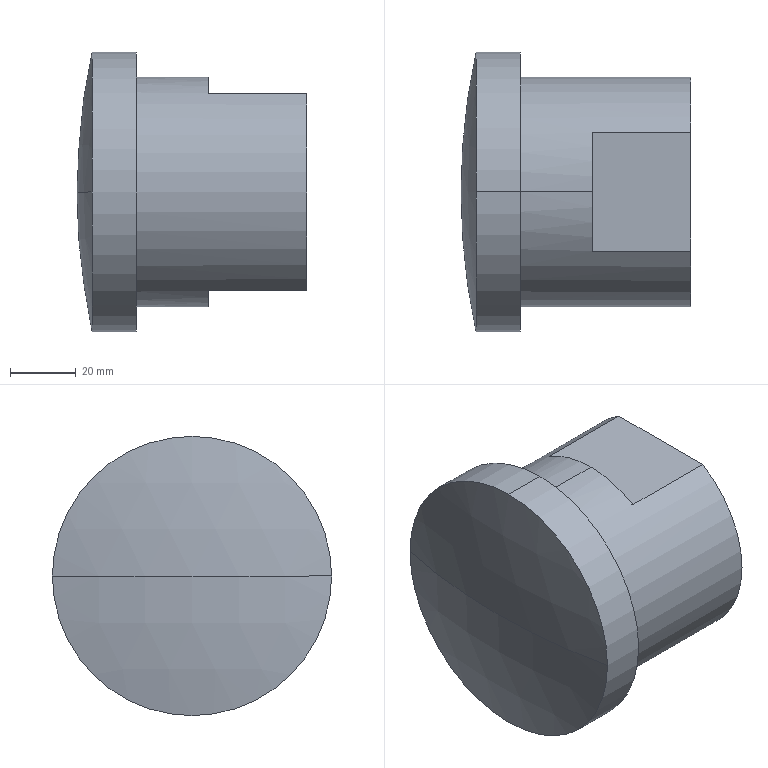Part | STEP file | OP10-027_cylinder connector (R) | 1 solid | 16 faces | box 70 x 85 x 85 mm | volume 228647 mm3 | cylinder 6 | plane 6 | cone 2 | sphere 2 | commonest cylinder face diameters 38.5 x2 70 x2 85 x2
STEP:
#1=CARTESIAN_POINT('',(0.,0.,0.));
#2=DIRECTION('',(0.,0.,1.));
#3=DIRECTION('',(1.,0.,0.));
#4=AXIS2_PLACEMENT_3D('',#1,#2,#3);
#5=CARTESIAN_POINT('',(-42.,0.,-19.25));
#6=VERTEX_POINT('',#5);
#7=CARTESIAN_POINT('',(0.,0.,-19.25));
#8=VERTEX_POINT('',#7);
#9=CARTESIAN_POINT('',(0.,0.,-19.25));
#10=DIRECTION('',(1.,0.,0.));
#11=VECTOR('',#10,1.);
#12=LINE('',#9,#11);
#13=CARTESIAN_POINT('',(0.,0.,0.));
#14=DIRECTION('',(1.,0.,0.));
#15=DIRECTION('',(0.,0.,-1.));
#16=AXIS2_PLACEMENT_3D('',#13,#14,#15);
#17=CYLINDRICAL_SURFACE('',#16,19.25);
#18=CARTESIAN_POINT('',(6.283,0.));
#19=DIRECTION('',(0.,1.));
#20=VECTOR('',#19,1.);
#21=LINE('',#18,#20);
#22=(GEOMETRIC_REPRESENTATION_CONTEXT(2)PARAMETRIC_REPRESENTATION_CONTEXT()REPRESENTATION_CONTEXT('',''));
#23=DEFINITIONAL_REPRESENTATION('',(#21),#22);
#24=PCURVE('',#17,#23);
#25=CARTESIAN_POINT('',(0.,0.,0.));
#26=DIRECTION('',(1.,0.,0.));
#27=DIRECTION('',(0.,0.,-1.));
#28=AXIS2_PLACEMENT_3D('',#25,#26,#27);
#29=CYLINDRICAL_SURFACE('',#28,19.25);
#30=CARTESIAN_POINT('',(0.,0.));
#31=DIRECTION('',(0.,1.));
#32=VECTOR('',#31,1.);
#33=LINE('',#30,#32);
#34=(GEOMETRIC_REPRESENTATION_CONTEXT(2)PARAMETRIC_REPRESENTATION_CONTEXT()REPRESENTATION_CONTEXT('',''));
#35=DEFINITIONAL_REPRESENTATION('',(#33),#34);
#36=PCURVE('',#29,#35);
#37=SURFACE_CURVE('',#12,(#24,#36),.PCURVE_S1.);
#38=EDGE_CURVE('',#6,#8,#37,.T.);
#39=ORIENTED_EDGE('',*,*,#38,.T.);
#40=CARTESIAN_POINT('',(0.,0.,19.25));
#41=VERTEX_POINT('',#40);
#42=CARTESIAN_POINT('',(0.,0.,0.));
#43=DIRECTION('',(1.,0.,0.));
#44=DIRECTION('',(0.,0.,-1.));
#45=AXIS2_PLACEMENT_3D('',#42,#43,#44);
#46=CIRCLE('',#45,19.25);
#47=CARTESIAN_POINT('',(0.,0.));
#48=DIRECTION('',(1.,0.));
#49=VECTOR('',#48,1.);
#50=LINE('',#47,#49);
#51=(GEOMETRIC_REPRESENTATION_CONTEXT(2)PARAMETRIC_REPRESENTATION_CONTEXT()REPRESENTATION_CONTEXT('',''));
#52=DEFINITIONAL_REPRESENTATION('',(#50),#51);
#53=PCURVE('',#17,#52);
#54=CARTESIAN_POINT('',(0.,0.,0.));
#55=DIRECTION('',(1.,0.,0.));
#56=DIRECTION('',(0.,0.,-1.));
#57=AXIS2_PLACEMENT_3D('',#54,#55,#56);
#58=PLANE('',#57);
#59=CARTESIAN_POINT('',(0.,0.));
#60=DIRECTION('',(1.,0.));
#61=AXIS2_PLACEMENT_2D('',#59,#60);
#62=CIRCLE('',#61,19.25);
#63=(GEOMETRIC_REPRESENTATION_CONTEXT(2)PARAMETRIC_REPRESENTATION_CONTEXT()REPRESENTATION_CONTEXT('',''));
#64=DEFINITIONAL_REPRESENTATION('',(#62),#63);
#65=PCURVE('',#58,#64);
#66=SURFACE_CURVE('',#46,(#53,#65),.PCURVE_S1.);
#67=EDGE_CURVE('',#41,#8,#66,.T.);
#68=ORIENTED_EDGE('',*,*,#67,.F.);
#69=CARTESIAN_POINT('',(-42.,0.,19.25));
#70=VERTEX_POINT('',#69);
#71=CARTESIAN_POINT('',(0.,0.,19.25));
#72=DIRECTION('',(1.,0.,0.));
#73=VECTOR('',#72,1.);
#74=LINE('',#71,#73);
#75=CARTESIAN_POINT('',(3.142,0.));
#76=DIRECTION('',(0.,1.));
#77=VECTOR('',#76,1.);
#78=LINE('',#75,#77);
#79=(GEOMETRIC_REPRESENTATION_CONTEXT(2)PARAMETRIC_REPRESENTATION_CONTEXT()REPRESENTATION_CONTEXT('',''));
#80=DEFINITIONAL_REPRESENTATION('',(#78),#79);
#81=PCURVE('',#17,#80);
#82=CARTESIAN_POINT('',(3.142,0.));
#83=DIRECTION('',(0.,1.));
#84=VECTOR('',#83,1.);
#85=LINE('',#82,#84);
#86=(GEOMETRIC_REPRESENTATION_CONTEXT(2)PARAMETRIC_REPRESENTATION_CONTEXT()REPRESENTATION_CONTEXT('',''));
#87=DEFINITIONAL_REPRESENTATION('',(#85),#86);
#88=PCURVE('',#29,#87);
#89=SURFACE_CURVE('',#74,(#81,#88),.PCURVE_S1.);
#90=EDGE_CURVE('',#70,#41,#89,.T.);
#91=ORIENTED_EDGE('',*,*,#90,.F.);
#92=CARTESIAN_POINT('',(-42.,0.,0.));
#93=DIRECTION('',(1.,0.,0.));
#94=DIRECTION('',(0.,0.,-1.));
#95=AXIS2_PLACEMENT_3D('',#92,#93,#94);
#96=CIRCLE('',#95,19.25);
#97=CARTESIAN_POINT('',(0.,-42.));
#98=DIRECTION('',(1.,0.));
#99=VECTOR('',#98,1.);
#100=LINE('',#97,#99);
#101=(GEOMETRIC_REPRESENTATION_CONTEXT(2)PARAMETRIC_REPRESENTATION_CONTEXT()REPRESENTATION_CONTEXT('',''));
#102=DEFINITIONAL_REPRESENTATION('',(#100),#101);
#103=PCURVE('',#17,#102);
#104=CARTESIAN_POINT('',(-42.,0.,0.));
#105=DIRECTION('',(1.,0.,0.));
#106=DIRECTION('',(0.,0.,-1.));
#107=AXIS2_PLACEMENT_3D('',#104,#105,#106);
#108=CONICAL_SURFACE('',#107,19.25,1.03);
#109=CARTESIAN_POINT('',(0.,0.));
#110=DIRECTION('',(1.,0.));
#111=VECTOR('',#110,1.);
#112=LINE('',#109,#111);
#113=(GEOMETRIC_REPRESENTATION_CONTEXT(2)PARAMETRIC_REPRESENTATION_CONTEXT()REPRESENTATION_CONTEXT('',''));
#114=DEFINITIONAL_REPRESENTATION('',(#112),#113);
#115=PCURVE('',#108,#114);
#116=SURFACE_CURVE('',#96,(#103,#115),.PCURVE_S1.);
#117=EDGE_CURVE('',#70,#6,#116,.T.);
#118=ORIENTED_EDGE('',*,*,#117,.T.);
#119=EDGE_LOOP('',(#39,#68,#91,#118));
#120=FACE_BOUND('',#119,.F.);
#121=ADVANCED_FACE('',(#120),#17,.F.);
#122=ORIENTED_EDGE('',*,*,#117,.F.);
#123=CARTESIAN_POINT('',(-53.567,0.,0.));
#124=VERTEX_POINT('',#123);
#125=CARTESIAN_POINT('',(-42.,0.,19.25));
#126=DIRECTION('',(0.515,0.,0.8572));
#127=VECTOR('',#126,1.);
#128=LINE('',#125,#127);
#129=CARTESIAN_POINT('',(3.142,0.));
#130=DIRECTION('',(0.,1.));
#131=VECTOR('',#130,1.);
#132=LINE('',#129,#131);
#133=(GEOMETRIC_REPRESENTATION_CONTEXT(2)PARAMETRIC_REPRESENTATION_CONTEXT()REPRESENTATION_CONTEXT('',''));
#134=DEFINITIONAL_REPRESENTATION('',(#132),#133);
#135=PCURVE('',#108,#134);
#136=CARTESIAN_POINT('',(-42.,0.,0.));
#137=DIRECTION('',(1.,0.,0.));
#138=DIRECTION('',(0.,0.,-1.));
#139=AXIS2_PLACEMENT_3D('',#136,#137,#138);
#140=CONICAL_SURFACE('',#139,19.25,1.03);
#141=CARTESIAN_POINT('',(3.142,0.));
#142=DIRECTION('',(0.,1.));
#143=VECTOR('',#142,1.);
#144=LINE('',#141,#143);
#145=(GEOMETRIC_REPRESENTATION_CONTEXT(2)PARAMETRIC_REPRESENTATION_CONTEXT()REPRESENTATION_CONTEXT('',''));
#146=DEFINITIONAL_REPRESENTATION('',(#144),#145);
#147=PCURVE('',#140,#146);
#148=SURFACE_CURVE('',#128,(#135,#147),.PCURVE_S1.);
#149=EDGE_CURVE('',#124,#70,#148,.T.);
#150=ORIENTED_EDGE('',*,*,#149,.F.);
#151=CARTESIAN_POINT('',(-42.,0.,-19.25));
#152=DIRECTION('',(0.515,0.,-0.8572));
#153=VECTOR('',#152,1.);
#154=LINE('',#151,#153);
#155=CARTESIAN_POINT('',(6.283,0.));
#156=DIRECTION('',(0.,1.));
#157=VECTOR('',#156,1.);
#158=LINE('',#155,#157);
#159=(GEOMETRIC_REPRESENTATION_CONTEXT(2)PARAMETRIC_REPRESENTATION_CONTEXT()REPRESENTATION_CONTEXT('',''));
#160=DEFINITIONAL_REPRESENTATION('',(#158),#159);
#161=PCURVE('',#108,#160);
#162=CARTESIAN_POINT('',(0.,0.));
#163=DIRECTION('',(0.,1.));
#164=VECTOR('',#163,1.);
#165=LINE('',#162,#164);
#166=(GEOMETRIC_REPRESENTATION_CONTEXT(2)PARAMETRIC_REPRESENTATION_CONTEXT()REPRESENTATION_CONTEXT('',''));
#167=DEFINITIONAL_REPRESENTATION('',(#165),#166);
#168=PCURVE('',#140,#167);
#169=SURFACE_CURVE('',#154,(#161,#168),.PCURVE_S1.);
#170=EDGE_CURVE('',#124,#6,#169,.T.);
#171=ORIENTED_EDGE('',*,*,#170,.T.);
#172=EDGE_LOOP('',(#122,#150,#171));
#173=FACE_BOUND('',#172,.F.);
#174=ADVANCED_FACE('',(#173),#108,.F.);
#175=CARTESIAN_POINT('',(-70.,0.,0.));
#176=VERTEX_POINT('',#175);
#177=CARTESIAN_POINT('',(-65.432,42.5,0.));
#178=VERTEX_POINT('',#177);
#179=CARTESIAN_POINT('',(130.,0.,0.));
#180=DIRECTION('',(0.,0.,-1.));
#181=DIRECTION('',(-1.,0.,0.));
#182=AXIS2_PLACEMENT_3D('',#179,#180,#181);
#183=CIRCLE('',#182,200.);
#184=CARTESIAN_POINT('',(130.,0.,0.));
#185=DIRECTION('',(0.,0.,1.));
#186=DIRECTION('',(0.,1.,0.));
#187=AXIS2_PLACEMENT_3D('',#184,#185,#186);
#188=SPHERICAL_SURFACE('',#187,200.);
#189=CARTESIAN_POINT('',(1.571,0.));
#190=DIRECTION('',(-1.,0.));
#191=VECTOR('',#190,1.);
#192=LINE('',#189,#191);
#193=(GEOMETRIC_REPRESENTATION_CONTEXT(2)PARAMETRIC_REPRESENTATION_CONTEXT()REPRESENTATION_CONTEXT('',''));
#194=DEFINITIONAL_REPRESENTATION('',(#192),#193);
#195=PCURVE('',#188,#194);
#196=CARTESIAN_POINT('',(130.,0.,0.));
#197=DIRECTION('',(0.,0.,1.));
#198=DIRECTION('',(0.,1.,0.));
#199=AXIS2_PLACEMENT_3D('',#196,#197,#198);
#200=SPHERICAL_SURFACE('',#199,200.);
#201=CARTESIAN_POINT('',(1.571,0.));
#202=DIRECTION('',(-1.,0.));
#203=VECTOR('',#202,1.);
#204=LINE('',#201,#203);
#205=(GEOMETRIC_REPRESENTATION_CONTEXT(2)PARAMETRIC_REPRESENTATION_CONTEXT()REPRESENTATION_CONTEXT('',''));
#206=DEFINITIONAL_REPRESENTATION('',(#204),#205);
#207=PCURVE('',#200,#206);
#208=SURFACE_CURVE('',#183,(#195,#207),.PCURVE_S1.);
#209=EDGE_CURVE('',#176,#178,#208,.T.);
#210=ORIENTED_EDGE('',*,*,#209,.F.);
#211=CARTESIAN_POINT('',(-65.432,-42.5,0.));
#212=VERTEX_POINT('',#211);
#213=CARTESIAN_POINT('',(130.,0.,0.));
#214=DIRECTION('',(0.,0.,1.));
#215=DIRECTION('',(0.,-1.,0.));
#216=AXIS2_PLACEMENT_3D('',#213,#214,#215);
#217=CIRCLE('',#216,200.);
#218=CARTESIAN_POINT('',(-3.142,0.));
#219=DIRECTION('',(1.,0.));
#220=VECTOR('',#219,1.);
#221=LINE('',#218,#220);
#222=(GEOMETRIC_REPRESENTATION_CONTEXT(2)PARAMETRIC_REPRESENTATION_CONTEXT()REPRESENTATION_CONTEXT('',''));
#223=DEFINITIONAL_REPRESENTATION('',(#221),#222);
#224=PCURVE('',#188,#223);
#225=CARTESIAN_POINT('',(-3.142,0.));
#226=DIRECTION('',(1.,0.));
#227=VECTOR('',#226,1.);
#228=LINE('',#225,#227);
#229=(GEOMETRIC_REPRESENTATION_CONTEXT(2)PARAMETRIC_REPRESENTATION_CONTEXT()REPRESENTATION_CONTEXT('',''));
#230=DEFINITIONAL_REPRESENTATION('',(#228),#229);
#231=PCURVE('',#200,#230);
#232=SURFACE_CURVE('',#217,(#224,#231),.PCURVE_S1.);
#233=EDGE_CURVE('',#176,#212,#232,.T.);
#234=ORIENTED_EDGE('',*,*,#233,.T.);
#235=CARTESIAN_POINT('',(-65.432,0.,42.5));
#236=VERTEX_POINT('',#235);
#237=CARTESIAN_POINT('',(-65.432,0.,0.));
#238=DIRECTION('',(1.,0.,0.));
#239=DIRECTION('',(0.,0.,-1.));
#240=AXIS2_PLACEMENT_3D('',#237,#238,#239);
#241=CIRCLE('',#240,42.5);
#242=CARTESIAN_POINT('',(1.571,0.2141));
#243=CARTESIAN_POINT('',(1.576,0.2141));
#244=CARTESIAN_POINT('',(1.586,0.2138));
#245=CARTESIAN_POINT('',(1.602,0.2121));
#246=CARTESIAN_POINT('',(1.617,0.2093));
#247=CARTESIAN_POINT('',(1.632,0.2055));
#248=CARTESIAN_POINT('',(1.647,0.2006));
#249=CARTESIAN_POINT('',(1.661,0.1947));
#250=CARTESIAN_POINT('',(1.675,0.1878));
#251=CARTESIAN_POINT('',(1.688,0.1799));
#252=CARTESIAN_POINT('',(1.701,0.1711));
#253=CARTESIAN_POINT('',(1.712,0.1614));
#254=CARTESIAN_POINT('',(1.724,0.151));
#255=CARTESIAN_POINT('',(1.734,0.1397));
#256=CARTESIAN_POINT('',(1.743,0.1278));
#257=CARTESIAN_POINT('',(1.752,0.1152));
#258=CARTESIAN_POINT('',(1.76,0.1021));
#259=CARTESIAN_POINT('',(1.766,0.08846));
#260=CARTESIAN_POINT('',(1.772,0.07439));
#261=CARTESIAN_POINT('',(1.777,0.05995));
#262=CARTESIAN_POINT('',(1.78,0.04522));
#263=CARTESIAN_POINT('',(1.783,0.03027));
#264=CARTESIAN_POINT('',(1.785,0.01517));
#265=CARTESIAN_POINT('',(1.785,0.005058));
#266=CARTESIAN_POINT('',(1.785,0.));
#267=B_SPLINE_CURVE_WITH_KNOTS('',3,(#242,#243,#244,#245,#246,#247,#248,#249,#250,#251,#252,#253,#254,#255,#256,#257,#258,#259,#260,#261,#262,#263,#264,#265,#266),.UNSPECIFIED.,.F.,.F.,(4,1,1,1,1,1,1,1,1,1,1,1,1,1,1,1,1,1,1,1,1,1,4),(3.142,3.213,3.284,3.356,3.427,3.499,3.57,3.641,3.713,3.784,3.856,3.927,3.998,4.07,4.141,4.213,4.284,4.355,4.427,4.498,4.57,4.641,4.712),.QUASI_UNIFORM_KNOTS.);
#268=(GEOMETRIC_REPRESENTATION_CONTEXT(2)PARAMETRIC_REPRESENTATION_CONTEXT()REPRESENTATION_CONTEXT('',''));
#269=DEFINITIONAL_REPRESENTATION('',(#267),#268);
#270=PCURVE('',#188,#269);
#271=CARTESIAN_POINT('',(0.,0.,0.));
#272=DIRECTION('',(1.,0.,0.));
#273=DIRECTION('',(0.,0.,-1.));
#274=AXIS2_PLACEMENT_3D('',#271,#272,#273);
#275=CYLINDRICAL_SURFACE('',#274,42.5);
#276=CARTESIAN_POINT('',(0.,-65.432));
#277=DIRECTION('',(1.,0.));
#278=VECTOR('',#277,1.);
#279=LINE('',#276,#278);
#280=(GEOMETRIC_REPRESENTATION_CONTEXT(2)PARAMETRIC_REPRESENTATION_CONTEXT()REPRESENTATION_CONTEXT('',''));
#281=DEFINITIONAL_REPRESENTATION('',(#279),#280);
#282=PCURVE('',#275,#281);
#283=SURFACE_CURVE('',#241,(#270,#282),.PCURVE_S1.);
#284=EDGE_CURVE('',#236,#212,#283,.T.);
#285=ORIENTED_EDGE('',*,*,#284,.F.);
#286=CARTESIAN_POINT('',(-65.432,0.,0.));
#287=DIRECTION('',(1.,0.,0.));
#288=DIRECTION('',(0.,0.,-1.));
#289=AXIS2_PLACEMENT_3D('',#286,#287,#288);
#290=CIRCLE('',#289,42.5);
#291=CARTESIAN_POINT('',(1.357,0.));
#292=CARTESIAN_POINT('',(1.357,0.005058));
#293=CARTESIAN_POINT('',(1.357,0.01517));
#294=CARTESIAN_POINT('',(1.359,0.03027));
#295=CARTESIAN_POINT('',(1.361,0.04522));
#296=CARTESIAN_POINT('',(1.365,0.05995));
#297=CARTESIAN_POINT('',(1.37,0.07439));
#298=CARTESIAN_POINT('',(1.375,0.08846));
#299=CARTESIAN_POINT('',(1.382,0.1021));
#300=CARTESIAN_POINT('',(1.39,0.1152));
#301=CARTESIAN_POINT('',(1.398,0.1278));
#302=CARTESIAN_POINT('',(1.408,0.1397));
#303=CARTESIAN_POINT('',(1.418,0.151));
#304=CARTESIAN_POINT('',(1.429,0.1614));
#305=CARTESIAN_POINT('',(1.441,0.1711));
#306=CARTESIAN_POINT('',(1.454,0.1799));
#307=CARTESIAN_POINT('',(1.467,0.1878));
#308=CARTESIAN_POINT('',(1.481,0.1947));
#309=CARTESIAN_POINT('',(1.495,0.2006));
#310=CARTESIAN_POINT('',(1.51,0.2055));
#311=CARTESIAN_POINT('',(1.525,0.2093));
#312=CARTESIAN_POINT('',(1.54,0.2121));
#313=CARTESIAN_POINT('',(1.555,0.2138));
#314=CARTESIAN_POINT('',(1.566,0.2141));
#315=CARTESIAN_POINT('',(1.571,0.2141));
#316=B_SPLINE_CURVE_WITH_KNOTS('',3,(#291,#292,#293,#294,#295,#296,#297,#298,#299,#300,#301,#302,#303,#304,#305,#306,#307,#308,#309,#310,#311,#312,#313,#314,#315),.UNSPECIFIED.,.F.,.F.,(4,1,1,1,1,1,1,1,1,1,1,1,1,1,1,1,1,1,1,1,1,1,4),(1.571,1.642,1.714,1.785,1.856,1.928,1.999,2.071,2.142,2.213,2.285,2.356,2.428,2.499,2.57,2.642,2.713,2.785,2.856,2.927,2.999,3.07,3.142),.QUASI_UNIFORM_KNOTS.);
#317=(GEOMETRIC_REPRESENTATION_CONTEXT(2)PARAMETRIC_REPRESENTATION_CONTEXT()REPRESENTATION_CONTEXT('',''));
#318=DEFINITIONAL_REPRESENTATION('',(#316),#317);
#319=PCURVE('',#188,#318);
#320=CARTESIAN_POINT('',(0.,0.,0.));
#321=DIRECTION('',(1.,0.,0.));
#322=DIRECTION('',(0.,0.,-1.));
#323=AXIS2_PLACEMENT_3D('',#320,#321,#322);
#324=CYLINDRICAL_SURFACE('',#323,42.5);
#325=CARTESIAN_POINT('',(0.,-65.432));
#326=DIRECTION('',(1.,0.));
#327=VECTOR('',#326,1.);
#328=LINE('',#325,#327);
#329=(GEOMETRIC_REPRESENTATION_CONTEXT(2)PARAMETRIC_REPRESENTATION_CONTEXT()REPRESENTATION_CONTEXT('',''));
#330=DEFINITIONAL_REPRESENTATION('',(#328),#329);
#331=PCURVE('',#324,#330);
#332=SURFACE_CURVE('',#290,(#319,#331),.PCURVE_S1.);
#333=EDGE_CURVE('',#178,#236,#332,.T.);
#334=ORIENTED_EDGE('',*,*,#333,.F.);
#335=EDGE_LOOP('',(#210,#234,#285,#334));
#336=FACE_BOUND('',#335,.T.);
#337=ADVANCED_FACE('',(#336),#188,.T.);
#338=CARTESIAN_POINT('',(-65.432,0.,-42.5));
#339=VERTEX_POINT('',#338);
#340=CARTESIAN_POINT('',(-65.432,0.,0.));
#341=DIRECTION('',(1.,0.,0.));
#342=DIRECTION('',(0.,0.,-1.));
#343=AXIS2_PLACEMENT_3D('',#340,#341,#342);
#344=CIRCLE('',#343,42.5);
#345=CARTESIAN_POINT('',(0.,-65.432));
#346=DIRECTION('',(1.,0.));
#347=VECTOR('',#346,1.);
#348=LINE('',#345,#347);
#349=(GEOMETRIC_REPRESENTATION_CONTEXT(2)PARAMETRIC_REPRESENTATION_CONTEXT()REPRESENTATION_CONTEXT('',''));
#350=DEFINITIONAL_REPRESENTATION('',(#348),#349);
#351=PCURVE('',#324,#350);
#352=CARTESIAN_POINT('',(1.571,-0.2141));
#353=CARTESIAN_POINT('',(1.566,-0.2141));
#354=CARTESIAN_POINT('',(1.555,-0.2138));
#355=CARTESIAN_POINT('',(1.54,-0.2121));
#356=CARTESIAN_POINT('',(1.525,-0.2093));
#357=CARTESIAN_POINT('',(1.51,-0.2055));
#358=CARTESIAN_POINT('',(1.495,-0.2006));
#359=CARTESIAN_POINT('',(1.481,-0.1947));
#360=CARTESIAN_POINT('',(1.467,-0.1878));
#361=CARTESIAN_POINT('',(1.454,-0.1799));
#362=CARTESIAN_POINT('',(1.441,-0.1711));
#363=CARTESIAN_POINT('',(1.429,-0.1614));
#364=CARTESIAN_POINT('',(1.418,-0.151));
#365=CARTESIAN_POINT('',(1.408,-0.1397));
#366=CARTESIAN_POINT('',(1.398,-0.1278));
#367=CARTESIAN_POINT('',(1.39,-0.1152));
#368=CARTESIAN_POINT('',(1.382,-0.1021));
#369=CARTESIAN_POINT('',(1.375,-0.08846));
#370=CARTESIAN_POINT('',(1.37,-0.07439));
#371=CARTESIAN_POINT('',(1.365,-0.05995));
#372=CARTESIAN_POINT('',(1.361,-0.04522));
#373=CARTESIAN_POINT('',(1.359,-0.03027));
#374=CARTESIAN_POINT('',(1.357,-0.01517));
#375=CARTESIAN_POINT('',(1.357,-0.005058));
#376=CARTESIAN_POINT('',(1.357,0.));
#377=B_SPLINE_CURVE_WITH_KNOTS('',3,(#352,#353,#354,#355,#356,#357,#358,#359,#360,#361,#362,#363,#364,#365,#366,#367,#368,#369,#370,#371,#372,#373,#374,#375,#376),.UNSPECIFIED.,.F.,.F.,(4,1,1,1,1,1,1,1,1,1,1,1,1,1,1,1,1,1,1,1,1,1,4),(0.,0.0714,0.1428,0.2142,0.2856,0.357,0.4284,0.4998,0.5712,0.6426,0.714,0.7854,0.8568,0.9282,0.9996,1.071,1.142,1.214,1.285,1.357,1.428,1.499,1.571),.QUASI_UNIFORM_KNOTS.);
#378=(GEOMETRIC_REPRESENTATION_CONTEXT(2)PARAMETRIC_REPRESENTATION_CONTEXT()REPRESENTATION_CONTEXT('',''));
#379=DEFINITIONAL_REPRESENTATION('',(#377),#378);
#380=PCURVE('',#200,#379);
#381=SURFACE_CURVE('',#344,(#351,#380),.PCURVE_S1.);
#382=EDGE_CURVE('',#339,#178,#381,.T.);
#383=ORIENTED_EDGE('',*,*,#382,.T.);
#384=ORIENTED_EDGE('',*,*,#333,.T.);
#385=CARTESIAN_POINT('',(-52.,0.,42.5));
#386=VERTEX_POINT('',#385);
#387=CARTESIAN_POINT('',(0.,0.,42.5));
#388=DIRECTION('',(1.,0.,0.));
#389=VECTOR('',#388,1.);
#390=LINE('',#387,#389);
#391=CARTESIAN_POINT('',(3.142,0.));
#392=DIRECTION('',(0.,1.));
#393=VECTOR('',#392,1.);
#394=LINE('',#391,#393);
#395=(GEOMETRIC_REPRESENTATION_CONTEXT(2)PARAMETRIC_REPRESENTATION_CONTEXT()REPRESENTATION_CONTEXT('',''));
#396=DEFINITIONAL_REPRESENTATION('',(#394),#395);
#397=PCURVE('',#324,#396);
#398=CARTESIAN_POINT('',(3.142,0.));
#399=DIRECTION('',(0.,1.));
#400=VECTOR('',#399,1.);
#401=LINE('',#398,#400);
#402=(GEOMETRIC_REPRESENTATION_CONTEXT(2)PARAMETRIC_REPRESENTATION_CONTEXT()REPRESENTATION_CONTEXT('',''));
#403=DEFINITIONAL_REPRESENTATION('',(#401),#402);
#404=PCURVE('',#275,#403);
#405=SURFACE_CURVE('',#390,(#397,#404),.PCURVE_S1.);
#406=EDGE_CURVE('',#236,#386,#405,.T.);
#407=ORIENTED_EDGE('',*,*,#406,.T.);
#408=CARTESIAN_POINT('',(-52.,0.,-42.5));
#409=VERTEX_POINT('',#408);
#410=CARTESIAN_POINT('',(-52.,0.,0.));
#411=DIRECTION('',(1.,0.,0.));
#412=DIRECTION('',(0.,0.,-1.));
#413=AXIS2_PLACEMENT_3D('',#410,#411,#412);
#414=CIRCLE('',#413,42.5);
#415=CARTESIAN_POINT('',(0.,-52.));
#416=DIRECTION('',(1.,0.));
#417=VECTOR('',#416,1.);
#418=LINE('',#415,#417);
#419=(GEOMETRIC_REPRESENTATION_CONTEXT(2)PARAMETRIC_REPRESENTATION_CONTEXT()REPRESENTATION_CONTEXT('',''));
#420=DEFINITIONAL_REPRESENTATION('',(#418),#419);
#421=PCURVE('',#324,#420);
#422=CARTESIAN_POINT('',(-52.,35.,0.));
#423=DIRECTION('',(1.,0.,0.));
#424=DIRECTION('',(0.,0.,-1.));
#425=AXIS2_PLACEMENT_3D('',#422,#423,#424);
#426=PLANE('',#425);
#427=CARTESIAN_POINT('',(0.,-35.));
#428=DIRECTION('',(1.,0.));
#429=AXIS2_PLACEMENT_2D('',#427,#428);
#430=CIRCLE('',#429,42.5);
#431=(GEOMETRIC_REPRESENTATION_CONTEXT(2)PARAMETRIC_REPRESENTATION_CONTEXT()REPRESENTATION_CONTEXT('',''));
#432=DEFINITIONAL_REPRESENTATION('',(#430),#431);
#433=PCURVE('',#426,#432);
#434=SURFACE_CURVE('',#414,(#421,#433),.PCURVE_S1.);
#435=EDGE_CURVE('',#409,#386,#434,.T.);
#436=ORIENTED_EDGE('',*,*,#435,.F.);
#437=CARTESIAN_POINT('',(0.,0.,-42.5));
#438=DIRECTION('',(1.,0.,0.));
#439=VECTOR('',#438,1.);
#440=LINE('',#437,#439);
#441=CARTESIAN_POINT('',(0.,0.));
#442=DIRECTION('',(0.,1.));
#443=VECTOR('',#442,1.);
#444=LINE('',#441,#443);
#445=(GEOMETRIC_REPRESENTATION_CONTEXT(2)PARAMETRIC_REPRESENTATION_CONTEXT()REPRESENTATION_CONTEXT('',''));
#446=DEFINITIONAL_REPRESENTATION('',(#444),#445);
#447=PCURVE('',#324,#446);
#448=CARTESIAN_POINT('',(6.283,0.));
#449=DIRECTION('',(0.,1.));
#450=VECTOR('',#449,1.);
#451=LINE('',#448,#450);
#452=(GEOMETRIC_REPRESENTATION_CONTEXT(2)PARAMETRIC_REPRESENTATION_CONTEXT()REPRESENTATION_CONTEXT('',''));
#453=DEFINITIONAL_REPRESENTATION('',(#451),#452);
#454=PCURVE('',#275,#453);
#455=SURFACE_CURVE('',#440,(#447,#454),.PCURVE_S1.);
#456=EDGE_CURVE('',#339,#409,#455,.T.);
#457=ORIENTED_EDGE('',*,*,#456,.F.);
#458=EDGE_LOOP('',(#383,#384,#407,#436,#457));
#459=FACE_BOUND('',#458,.T.);
#460=ADVANCED_FACE('',(#459),#324,.T.);
#461=CARTESIAN_POINT('',(-52.,0.,-35.));
#462=VERTEX_POINT('',#461);
#463=CARTESIAN_POINT('',(-52.,0.,35.));
#464=VERTEX_POINT('',#463);
#465=CARTESIAN_POINT('',(-52.,0.,0.));
#466=DIRECTION('',(1.,0.,0.));
#467=DIRECTION('',(0.,0.,-1.));
#468=AXIS2_PLACEMENT_3D('',#465,#466,#467);
#469=CIRCLE('',#468,35.);
#470=CARTESIAN_POINT('',(0.,0.,0.));
#471=DIRECTION('',(1.,0.,0.));
#472=DIRECTION('',(0.,0.,-1.));
#473=AXIS2_PLACEMENT_3D('',#470,#471,#472);
#474=CYLINDRICAL_SURFACE('',#473,35.);
#475=CARTESIAN_POINT('',(0.,-52.));
#476=DIRECTION('',(1.,0.));
#477=VECTOR('',#476,1.);
#478=LINE('',#475,#477);
#479=(GEOMETRIC_REPRESENTATION_CONTEXT(2)PARAMETRIC_REPRESENTATION_CONTEXT()REPRESENTATION_CONTEXT('',''));
#480=DEFINITIONAL_REPRESENTATION('',(#478),#479);
#481=PCURVE('',#474,#480);
#482=CARTESIAN_POINT('',(0.,-35.));
#483=DIRECTION('',(1.,0.));
#484=AXIS2_PLACEMENT_2D('',#482,#483);
#485=CIRCLE('',#484,35.);
#486=(GEOMETRIC_REPRESENTATION_CONTEXT(2)PARAMETRIC_REPRESENTATION_CONTEXT()REPRESENTATION_CONTEXT('',''));
#487=DEFINITIONAL_REPRESENTATION('',(#485),#486);
#488=PCURVE('',#426,#487);
#489=SURFACE_CURVE('',#469,(#481,#488),.PCURVE_S1.);
#490=EDGE_CURVE('',#462,#464,#489,.T.);
#491=ORIENTED_EDGE('',*,*,#490,.T.);
#492=CARTESIAN_POINT('',(-30.,0.,35.));
#493=VERTEX_POINT('',#492);
#494=CARTESIAN_POINT('',(0.,0.,35.));
#495=DIRECTION('',(1.,0.,0.));
#496=VECTOR('',#495,1.);
#497=LINE('',#494,#496);
#498=CARTESIAN_POINT('',(3.142,0.));
#499=DIRECTION('',(0.,1.));
#500=VECTOR('',#499,1.);
#501=LINE('',#498,#500);
#502=(GEOMETRIC_REPRESENTATION_CONTEXT(2)PARAMETRIC_REPRESENTATION_CONTEXT()REPRESENTATION_CONTEXT('',''));
#503=DEFINITIONAL_REPRESENTATION('',(#501),#502);
#504=PCURVE('',#474,#503);
#505=CARTESIAN_POINT('',(0.,0.,0.));
#506=DIRECTION('',(1.,0.,0.));
#507=DIRECTION('',(0.,0.,-1.));
#508=AXIS2_PLACEMENT_3D('',#505,#506,#507);
#509=CYLINDRICAL_SURFACE('',#508,35.);
#510=CARTESIAN_POINT('',(3.142,0.));
#511=DIRECTION('',(0.,1.));
#512=VECTOR('',#511,1.);
#513=LINE('',#510,#512);
#514=(GEOMETRIC_REPRESENTATION_CONTEXT(2)PARAMETRIC_REPRESENTATION_CONTEXT()REPRESENTATION_CONTEXT('',''));
#515=DEFINITIONAL_REPRESENTATION('',(#513),#514);
#516=PCURVE('',#509,#515);
#517=SURFACE_CURVE('',#497,(#504,#516),.PCURVE_S1.);
#518=EDGE_CURVE('',#464,#493,#517,.T.);
#519=ORIENTED_EDGE('',*,*,#518,.T.);
#520=CARTESIAN_POINT('',(-30.,18.028,30.));
#521=VERTEX_POINT('',#520);
#522=CARTESIAN_POINT('',(-30.,0.,0.));
#523=DIRECTION('',(-1.,0.,0.));
#524=DIRECTION('',(0.,0.,-1.));
#525=AXIS2_PLACEMENT_3D('',#522,#523,#524);
#526=CIRCLE('',#525,35.);
#527=CARTESIAN_POINT('',(6.283,-30.));
#528=DIRECTION('',(-1.,0.));
#529=VECTOR('',#528,1.);
#530=LINE('',#527,#529);
#531=(GEOMETRIC_REPRESENTATION_CONTEXT(2)PARAMETRIC_REPRESENTATION_CONTEXT()REPRESENTATION_CONTEXT('',''));
#532=DEFINITIONAL_REPRESENTATION('',(#530),#531);
#533=PCURVE('',#474,#532);
#534=CARTESIAN_POINT('',(-30.,-35.,40.));
#535=DIRECTION('',(1.,0.,0.));
#536=DIRECTION('',(0.,0.,-1.));
#537=AXIS2_PLACEMENT_3D('',#534,#535,#536);
#538=PLANE('',#537);
#539=CARTESIAN_POINT('',(75.,35.));
#540=CARTESIAN_POINT('',(75.,-25.622));
#541=CARTESIAN_POINT('',(22.5,4.689));
#542=CARTESIAN_POINT('',(-30.,35.));
#543=CARTESIAN_POINT('',(22.5,65.311));
#544=CARTESIAN_POINT('',(75.,95.622));
#545=CARTESIAN_POINT('',(75.,35.));
#546=(BOUNDED_CURVE()B_SPLINE_CURVE(2,(#539,#540,#541,#542,#543,#544,#545),.UNSPECIFIED.,.T.,.F.)B_SPLINE_CURVE_WITH_KNOTS((1,2,2,2,2,1),(-2.094,0.,2.094,4.189,6.283,8.378),.UNSPECIFIED.)CURVE()GEOMETRIC_REPRESENTATION_ITEM()RATIONAL_B_SPLINE_CURVE((1.,0.5,1.,0.5,1.,0.5,1.))REPRESENTATION_ITEM(''));
#547=(GEOMETRIC_REPRESENTATION_CONTEXT(2)PARAMETRIC_REPRESENTATION_CONTEXT()REPRESENTATION_CONTEXT('',''));
#548=DEFINITIONAL_REPRESENTATION('',(#546),#547);
#549=PCURVE('',#538,#548);
#550=SURFACE_CURVE('',#526,(#533,#549),.PCURVE_S1.);
#551=EDGE_CURVE('',#493,#521,#550,.T.);
#552=ORIENTED_EDGE('',*,*,#551,.T.);
#553=CARTESIAN_POINT('',(0.,18.028,30.));
#554=VERTEX_POINT('',#553);
#555=CARTESIAN_POINT('',(0.,18.028,30.));
#556=DIRECTION('',(-1.,0.,0.));
#557=VECTOR('',#556,1.);
#558=LINE('',#555,#557);
#559=CARTESIAN_POINT('',(2.6,0.));
#560=DIRECTION('',(0.,-1.));
#561=VECTOR('',#560,1.);
#562=LINE('',#559,#561);
#563=(GEOMETRIC_REPRESENTATION_CONTEXT(2)PARAMETRIC_REPRESENTATION_CONTEXT()REPRESENTATION_CONTEXT('',''));
#564=DEFINITIONAL_REPRESENTATION('',(#562),#563);
#565=PCURVE('',#474,#564);
#566=CARTESIAN_POINT('',(0.,0.,30.));
#567=DIRECTION('',(0.,0.,-1.));
#568=DIRECTION('',(-1.,0.,0.));
#569=AXIS2_PLACEMENT_3D('',#566,#567,#568);
#570=PLANE('',#569);
#571=CARTESIAN_POINT('',(0.,18.028));
#572=DIRECTION('',(1.,0.));
#573=VECTOR('',#572,1.);
#574=LINE('',#571,#573);
#575=(GEOMETRIC_REPRESENTATION_CONTEXT(2)PARAMETRIC_REPRESENTATION_CONTEXT()REPRESENTATION_CONTEXT('',''));
#576=DEFINITIONAL_REPRESENTATION('',(#574),#575);
#577=PCURVE('',#570,#576);
#578=SURFACE_CURVE('',#558,(#565,#577),.PCURVE_S1.);
#579=EDGE_CURVE('',#554,#521,#578,.T.);
#580=ORIENTED_EDGE('',*,*,#579,.F.);
#581=CARTESIAN_POINT('',(0.,18.028,-30.));
#582=VERTEX_POINT('',#581);
#583=CARTESIAN_POINT('',(0.,0.,0.));
#584=DIRECTION('',(1.,0.,0.));
#585=DIRECTION('',(0.,0.,-1.));
#586=AXIS2_PLACEMENT_3D('',#583,#584,#585);
#587=CIRCLE('',#586,35.);
#588=CARTESIAN_POINT('',(0.,0.));
#589=DIRECTION('',(1.,0.));
#590=VECTOR('',#589,1.);
#591=LINE('',#588,#590);
#592=(GEOMETRIC_REPRESENTATION_CONTEXT(2)PARAMETRIC_REPRESENTATION_CONTEXT()REPRESENTATION_CONTEXT('',''));
#593=DEFINITIONAL_REPRESENTATION('',(#591),#592);
#594=PCURVE('',#474,#593);
#595=CARTESIAN_POINT('',(0.,0.));
#596=DIRECTION('',(1.,0.));
#597=AXIS2_PLACEMENT_2D('',#595,#596);
#598=CIRCLE('',#597,35.);
#599=(GEOMETRIC_REPRESENTATION_CONTEXT(2)PARAMETRIC_REPRESENTATION_CONTEXT()REPRESENTATION_CONTEXT('',''));
#600=DEFINITIONAL_REPRESENTATION('',(#598),#599);
#601=PCURVE('',#58,#600);
#602=SURFACE_CURVE('',#587,(#594,#601),.PCURVE_S1.);
#603=EDGE_CURVE('',#582,#554,#602,.T.);
#604=ORIENTED_EDGE('',*,*,#603,.F.);
#605=CARTESIAN_POINT('',(-30.,18.028,-30.));
#606=VERTEX_POINT('',#605);
#607=CARTESIAN_POINT('',(0.,18.028,-30.));
#608=DIRECTION('',(1.,0.,0.));
#609=VECTOR('',#608,1.);
#610=LINE('',#607,#609);
#611=CARTESIAN_POINT('',(0.5411,0.));
#612=DIRECTION('',(0.,1.));
#613=VECTOR('',#612,1.);
#614=LINE('',#611,#613);
#615=(GEOMETRIC_REPRESENTATION_CONTEXT(2)PARAMETRIC_REPRESENTATION_CONTEXT()REPRESENTATION_CONTEXT('',''));
#616=DEFINITIONAL_REPRESENTATION('',(#614),#615);
#617=PCURVE('',#474,#616);
#618=CARTESIAN_POINT('',(0.,0.,-30.));
#619=DIRECTION('',(0.,0.,1.));
#620=DIRECTION('',(-1.,0.,0.));
#621=AXIS2_PLACEMENT_3D('',#618,#619,#620);
#622=PLANE('',#621);
#623=CARTESIAN_POINT('',(0.,-18.028));
#624=DIRECTION('',(-1.,0.));
#625=VECTOR('',#624,1.);
#626=LINE('',#623,#625);
#627=(GEOMETRIC_REPRESENTATION_CONTEXT(2)PARAMETRIC_REPRESENTATION_CONTEXT()REPRESENTATION_CONTEXT('',''));
#628=DEFINITIONAL_REPRESENTATION('',(#626),#627);
#629=PCURVE('',#622,#628);
#630=SURFACE_CURVE('',#610,(#617,#629),.PCURVE_S1.);
#631=EDGE_CURVE('',#606,#582,#630,.T.);
#632=ORIENTED_EDGE('',*,*,#631,.F.);
#633=CARTESIAN_POINT('',(-30.,0.,-35.));
#634=VERTEX_POINT('',#633);
#635=CARTESIAN_POINT('',(-30.,0.,0.));
#636=DIRECTION('',(1.,0.,0.));
#637=DIRECTION('',(0.,0.,1.));
#638=AXIS2_PLACEMENT_3D('',#635,#636,#637);
#639=CIRCLE('',#638,35.);
#640=CARTESIAN_POINT('',(-3.142,-30.));
#641=DIRECTION('',(1.,0.));
#642=VECTOR('',#641,1.);
#643=LINE('',#640,#642);
#644=(GEOMETRIC_REPRESENTATION_CONTEXT(2)PARAMETRIC_REPRESENTATION_CONTEXT()REPRESENTATION_CONTEXT('',''));
#645=DEFINITIONAL_REPRESENTATION('',(#643),#644);
#646=PCURVE('',#474,#645);
#647=CARTESIAN_POINT('',(-30.,-35.,-40.));
#648=DIRECTION('',(-1.,0.,0.));
#649=DIRECTION('',(0.,0.,1.));
#650=AXIS2_PLACEMENT_3D('',#647,#648,#649);
#651=PLANE('',#650);
#652=CARTESIAN_POINT('',(75.,35.));
#653=CARTESIAN_POINT('',(75.,-25.622));
#654=CARTESIAN_POINT('',(22.5,4.689));
#655=CARTESIAN_POINT('',(-30.,35.));
#656=CARTESIAN_POINT('',(22.5,65.311));
#657=CARTESIAN_POINT('',(75.,95.622));
#658=CARTESIAN_POINT('',(75.,35.));
#659=(BOUNDED_CURVE()B_SPLINE_CURVE(2,(#652,#653,#654,#655,#656,#657,#658),.UNSPECIFIED.,.T.,.F.)B_SPLINE_CURVE_WITH_KNOTS((1,2,2,2,2,1),(-2.094,0.,2.094,4.189,6.283,8.378),.UNSPECIFIED.)CURVE()GEOMETRIC_REPRESENTATION_ITEM()RATIONAL_B_SPLINE_CURVE((1.,0.5,1.,0.5,1.,0.5,1.))REPRESENTATION_ITEM(''));
#660=(GEOMETRIC_REPRESENTATION_CONTEXT(2)PARAMETRIC_REPRESENTATION_CONTEXT()REPRESENTATION_CONTEXT('',''));
#661=DEFINITIONAL_REPRESENTATION('',(#659),#660);
#662=PCURVE('',#651,#661);
#663=SURFACE_CURVE('',#639,(#646,#662),.PCURVE_S1.);
#664=EDGE_CURVE('',#634,#606,#663,.T.);
#665=ORIENTED_EDGE('',*,*,#664,.F.);
#666=CARTESIAN_POINT('',(0.,0.,-35.));
#667=DIRECTION('',(1.,0.,0.));
#668=VECTOR('',#667,1.);
#669=LINE('',#666,#668);
#670=CARTESIAN_POINT('',(0.,0.));
#671=DIRECTION('',(0.,1.));
#672=VECTOR('',#671,1.);
#673=LINE('',#670,#672);
#674=(GEOMETRIC_REPRESENTATION_CONTEXT(2)PARAMETRIC_REPRESENTATION_CONTEXT()REPRESENTATION_CONTEXT('',''));
#675=DEFINITIONAL_REPRESENTATION('',(#673),#674);
#676=PCURVE('',#474,#675);
#677=CARTESIAN_POINT('',(6.283,0.));
#678=DIRECTION('',(0.,1.));
#679=VECTOR('',#678,1.);
#680=LINE('',#677,#679);
#681=(GEOMETRIC_REPRESENTATION_CONTEXT(2)PARAMETRIC_REPRESENTATION_CONTEXT()REPRESENTATION_CONTEXT('',''));
#682=DEFINITIONAL_REPRESENTATION('',(#680),#681);
#683=PCURVE('',#509,#682);
#684=SURFACE_CURVE('',#669,(#676,#683),.PCURVE_S1.);
#685=EDGE_CURVE('',#462,#634,#684,.T.);
#686=ORIENTED_EDGE('',*,*,#685,.F.);
#687=EDGE_LOOP('',(#491,#519,#552,#580,#604,#632,#665,#686));
#688=FACE_BOUND('',#687,.T.);
#689=ADVANCED_FACE('',(#688),#474,.T.);
#690=CARTESIAN_POINT('',(0.,0.,0.));
#691=DIRECTION('',(1.,0.,0.));
#692=DIRECTION('',(0.,0.,-1.));
#693=AXIS2_PLACEMENT_3D('',#690,#691,#692);
#694=CIRCLE('',#693,19.25);
#695=CARTESIAN_POINT('',(0.,0.));
#696=DIRECTION('',(1.,0.));
#697=AXIS2_PLACEMENT_2D('',#695,#696);
#698=CIRCLE('',#697,19.25);
#699=(GEOMETRIC_REPRESENTATION_CONTEXT(2)PARAMETRIC_REPRESENTATION_CONTEXT()REPRESENTATION_CONTEXT('',''));
#700=DEFINITIONAL_REPRESENTATION('',(#698),#699);
#701=PCURVE('',#58,#700);
#702=CARTESIAN_POINT('',(0.,0.));
#703=DIRECTION('',(1.,0.));
#704=VECTOR('',#703,1.);
#705=LINE('',#702,#704);
#706=(GEOMETRIC_REPRESENTATION_CONTEXT(2)PARAMETRIC_REPRESENTATION_CONTEXT()REPRESENTATION_CONTEXT('',''));
#707=DEFINITIONAL_REPRESENTATION('',(#705),#706);
#708=PCURVE('',#29,#707);
#709=SURFACE_CURVE('',#694,(#701,#708),.PCURVE_S1.);
#710=EDGE_CURVE('',#8,#41,#709,.T.);
#711=ORIENTED_EDGE('',*,*,#710,.F.);
#712=ORIENTED_EDGE('',*,*,#67,.F.);
#713=EDGE_LOOP('',(#711,#712));
#714=FACE_BOUND('',#713,.T.);
#715=CARTESIAN_POINT('',(0.,-18.028,-30.));
#716=VERTEX_POINT('',#715);
#717=CARTESIAN_POINT('',(0.,0.,-30.));
#718=DIRECTION('',(0.,-1.,0.));
#719=VECTOR('',#718,1.);
#720=LINE('',#717,#719);
#721=CARTESIAN_POINT('',(30.,0.));
#722=DIRECTION('',(0.,-1.));
#723=VECTOR('',#722,1.);
#724=LINE('',#721,#723);
#725=(GEOMETRIC_REPRESENTATION_CONTEXT(2)PARAMETRIC_REPRESENTATION_CONTEXT()REPRESENTATION_CONTEXT('',''));
#726=DEFINITIONAL_REPRESENTATION('',(#724),#725);
#727=PCURVE('',#58,#726);
#728=CARTESIAN_POINT('',(0.,0.));
#729=DIRECTION('',(0.,1.));
#730=VECTOR('',#729,1.);
#731=LINE('',#728,#730);
#732=(GEOMETRIC_REPRESENTATION_CONTEXT(2)PARAMETRIC_REPRESENTATION_CONTEXT()REPRESENTATION_CONTEXT('',''));
#733=DEFINITIONAL_REPRESENTATION('',(#731),#732);
#734=PCURVE('',#622,#733);
#735=SURFACE_CURVE('',#720,(#727,#734),.PCURVE_S1.);
#736=EDGE_CURVE('',#582,#716,#735,.T.);
#737=ORIENTED_EDGE('',*,*,#736,.F.);
#738=ORIENTED_EDGE('',*,*,#603,.T.);
#739=CARTESIAN_POINT('',(0.,-18.028,30.));
#740=VERTEX_POINT('',#739);
#741=CARTESIAN_POINT('',(0.,0.,30.));
#742=DIRECTION('',(0.,1.,0.));
#743=VECTOR('',#742,1.);
#744=LINE('',#741,#743);
#745=CARTESIAN_POINT('',(-30.,0.));
#746=DIRECTION('',(0.,1.));
#747=VECTOR('',#746,1.);
#748=LINE('',#745,#747);
#749=(GEOMETRIC_REPRESENTATION_CONTEXT(2)PARAMETRIC_REPRESENTATION_CONTEXT()REPRESENTATION_CONTEXT('',''));
#750=DEFINITIONAL_REPRESENTATION('',(#748),#749);
#751=PCURVE('',#58,#750);
#752=CARTESIAN_POINT('',(0.,0.));
#753=DIRECTION('',(0.,1.));
#754=VECTOR('',#753,1.);
#755=LINE('',#752,#754);
#756=(GEOMETRIC_REPRESENTATION_CONTEXT(2)PARAMETRIC_REPRESENTATION_CONTEXT()REPRESENTATION_CONTEXT('',''));
#757=DEFINITIONAL_REPRESENTATION('',(#755),#756);
#758=PCURVE('',#570,#757);
#759=SURFACE_CURVE('',#744,(#751,#758),.PCURVE_S1.);
#760=EDGE_CURVE('',#740,#554,#759,.T.);
#761=ORIENTED_EDGE('',*,*,#760,.F.);
#762=CARTESIAN_POINT('',(0.,0.,0.));
#763=DIRECTION('',(1.,0.,0.));
#764=DIRECTION('',(0.,0.,-1.));
#765=AXIS2_PLACEMENT_3D('',#762,#763,#764);
#766=CIRCLE('',#765,35.);
#767=CARTESIAN_POINT('',(0.,0.));
#768=DIRECTION('',(1.,0.));
#769=AXIS2_PLACEMENT_2D('',#767,#768);
#770=CIRCLE('',#769,35.);
#771=(GEOMETRIC_REPRESENTATION_CONTEXT(2)PARAMETRIC_REPRESENTATION_CONTEXT()REPRESENTATION_CONTEXT('',''));
#772=DEFINITIONAL_REPRESENTATION('',(#770),#771);
#773=PCURVE('',#58,#772);
#774=CARTESIAN_POINT('',(0.,0.));
#775=DIRECTION('',(1.,0.));
#776=VECTOR('',#775,1.);
#777=LINE('',#774,#776);
#778=(GEOMETRIC_REPRESENTATION_CONTEXT(2)PARAMETRIC_REPRESENTATION_CONTEXT()REPRESENTATION_CONTEXT('',''));
#779=DEFINITIONAL_REPRESENTATION('',(#777),#778);
#780=PCURVE('',#509,#779);
#781=SURFACE_CURVE('',#766,(#773,#780),.PCURVE_S1.);
#782=EDGE_CURVE('',#740,#716,#781,.T.);
#783=ORIENTED_EDGE('',*,*,#782,.T.);
#784=EDGE_LOOP('',(#737,#738,#761,#783));
#785=FACE_BOUND('',#784,.T.);
#786=ADVANCED_FACE('',(#714,#785),#58,.T.);
#787=ORIENTED_EDGE('',*,*,#518,.F.);
#788=CARTESIAN_POINT('',(-52.,0.,0.));
#789=DIRECTION('',(1.,0.,0.));
#790=DIRECTION('',(0.,0.,-1.));
#791=AXIS2_PLACEMENT_3D('',#788,#789,#790);
#792=CIRCLE('',#791,35.);
#793=CARTESIAN_POINT('',(0.,-52.));
#794=DIRECTION('',(1.,0.));
#795=VECTOR('',#794,1.);
#796=LINE('',#793,#795);
#797=(GEOMETRIC_REPRESENTATION_CONTEXT(2)PARAMETRIC_REPRESENTATION_CONTEXT()REPRESENTATION_CONTEXT('',''));
#798=DEFINITIONAL_REPRESENTATION('',(#796),#797);
#799=PCURVE('',#509,#798);
#800=CARTESIAN_POINT('',(0.,-35.));
#801=DIRECTION('',(1.,0.));
#802=AXIS2_PLACEMENT_2D('',#800,#801);
#803=CIRCLE('',#802,35.);
#804=(GEOMETRIC_REPRESENTATION_CONTEXT(2)PARAMETRIC_REPRESENTATION_CONTEXT()REPRESENTATION_CONTEXT('',''));
#805=DEFINITIONAL_REPRESENTATION('',(#803),#804);
#806=PCURVE('',#426,#805);
#807=SURFACE_CURVE('',#792,(#799,#806),.PCURVE_S1.);
#808=EDGE_CURVE('',#464,#462,#807,.T.);
#809=ORIENTED_EDGE('',*,*,#808,.T.);
#810=ORIENTED_EDGE('',*,*,#685,.T.);
#811=CARTESIAN_POINT('',(-30.,-18.028,-30.));
#812=VERTEX_POINT('',#811);
#813=CARTESIAN_POINT('',(-30.,0.,0.));
#814=DIRECTION('',(1.,0.,0.));
#815=DIRECTION('',(0.,0.,1.));
#816=AXIS2_PLACEMENT_3D('',#813,#814,#815);
#817=CIRCLE('',#816,35.);
#818=CARTESIAN_POINT('',(3.142,-30.));
#819=DIRECTION('',(1.,0.));
#820=VECTOR('',#819,1.);
#821=LINE('',#818,#820);
#822=(GEOMETRIC_REPRESENTATION_CONTEXT(2)PARAMETRIC_REPRESENTATION_CONTEXT()REPRESENTATION_CONTEXT('',''));
#823=DEFINITIONAL_REPRESENTATION('',(#821),#822);
#824=PCURVE('',#509,#823);
#825=CARTESIAN_POINT('',(75.,35.));
#826=CARTESIAN_POINT('',(75.,-25.622));
#827=CARTESIAN_POINT('',(22.5,4.689));
#828=CARTESIAN_POINT('',(-30.,35.));
#829=CARTESIAN_POINT('',(22.5,65.311));
#830=CARTESIAN_POINT('',(75.,95.622));
#831=CARTESIAN_POINT('',(75.,35.));
#832=(BOUNDED_CURVE()B_SPLINE_CURVE(2,(#825,#826,#827,#828,#829,#830,#831),.UNSPECIFIED.,.T.,.F.)B_SPLINE_CURVE_WITH_KNOTS((1,2,2,2,2,1),(-2.094,0.,2.094,4.189,6.283,8.378),.UNSPECIFIED.)CURVE()GEOMETRIC_REPRESENTATION_ITEM()RATIONAL_B_SPLINE_CURVE((1.,0.5,1.,0.5,1.,0.5,1.))REPRESENTATION_ITEM(''));
#833=(GEOMETRIC_REPRESENTATION_CONTEXT(2)PARAMETRIC_REPRESENTATION_CONTEXT()REPRESENTATION_CONTEXT('',''));
#834=DEFINITIONAL_REPRESENTATION('',(#832),#833);
#835=PCURVE('',#651,#834);
#836=SURFACE_CURVE('',#817,(#824,#835),.PCURVE_S1.);
#837=EDGE_CURVE('',#812,#634,#836,.T.);
#838=ORIENTED_EDGE('',*,*,#837,.F.);
#839=CARTESIAN_POINT('',(0.,-18.028,-30.));
#840=DIRECTION('',(-1.,0.,0.));
#841=VECTOR('',#840,1.);
#842=LINE('',#839,#841);
#843=CARTESIAN_POINT('',(5.742,0.));
#844=DIRECTION('',(0.,-1.));
#845=VECTOR('',#844,1.);
#846=LINE('',#843,#845);
#847=(GEOMETRIC_REPRESENTATION_CONTEXT(2)PARAMETRIC_REPRESENTATION_CONTEXT()REPRESENTATION_CONTEXT('',''));
#848=DEFINITIONAL_REPRESENTATION('',(#846),#847);
#849=PCURVE('',#509,#848);
#850=CARTESIAN_POINT('',(0.,18.028));
#851=DIRECTION('',(1.,0.));
#852=VECTOR('',#851,1.);
#853=LINE('',#850,#852);
#854=(GEOMETRIC_REPRESENTATION_CONTEXT(2)PARAMETRIC_REPRESENTATION_CONTEXT()REPRESENTATION_CONTEXT('',''));
#855=DEFINITIONAL_REPRESENTATION('',(#853),#854);
#856=PCURVE('',#622,#855);
#857=SURFACE_CURVE('',#842,(#849,#856),.PCURVE_S1.);
#858=EDGE_CURVE('',#716,#812,#857,.T.);
#859=ORIENTED_EDGE('',*,*,#858,.F.);
#860=ORIENTED_EDGE('',*,*,#782,.F.);
#861=CARTESIAN_POINT('',(-30.,-18.028,30.));
#862=VERTEX_POINT('',#861);
#863=CARTESIAN_POINT('',(0.,-18.028,30.));
#864=DIRECTION('',(1.,0.,0.));
#865=VECTOR('',#864,1.);
#866=LINE('',#863,#865);
#867=CARTESIAN_POINT('',(3.683,0.));
#868=DIRECTION('',(0.,1.));
#869=VECTOR('',#868,1.);
#870=LINE('',#867,#869);
#871=(GEOMETRIC_REPRESENTATION_CONTEXT(2)PARAMETRIC_REPRESENTATION_CONTEXT()REPRESENTATION_CONTEXT('',''));
#872=DEFINITIONAL_REPRESENTATION('',(#870),#871);
#873=PCURVE('',#509,#872);
#874=CARTESIAN_POINT('',(0.,-18.028));
#875=DIRECTION('',(-1.,0.));
#876=VECTOR('',#875,1.);
#877=LINE('',#874,#876);
#878=(GEOMETRIC_REPRESENTATION_CONTEXT(2)PARAMETRIC_REPRESENTATION_CONTEXT()REPRESENTATION_CONTEXT('',''));
#879=DEFINITIONAL_REPRESENTATION('',(#877),#878);
#880=PCURVE('',#570,#879);
#881=SURFACE_CURVE('',#866,(#873,#880),.PCURVE_S1.);
#882=EDGE_CURVE('',#862,#740,#881,.T.);
#883=ORIENTED_EDGE('',*,*,#882,.F.);
#884=CARTESIAN_POINT('',(-30.,0.,0.));
#885=DIRECTION('',(-1.,0.,0.));
#886=DIRECTION('',(0.,0.,-1.));
#887=AXIS2_PLACEMENT_3D('',#884,#885,#886);
#888=CIRCLE('',#887,35.);
#889=CARTESIAN_POINT('',(6.283,-30.));
#890=DIRECTION('',(-1.,0.));
#891=VECTOR('',#890,1.);
#892=LINE('',#889,#891);
#893=(GEOMETRIC_REPRESENTATION_CONTEXT(2)PARAMETRIC_REPRESENTATION_CONTEXT()REPRESENTATION_CONTEXT('',''));
#894=DEFINITIONAL_REPRESENTATION('',(#892),#893);
#895=PCURVE('',#509,#894);
#896=CARTESIAN_POINT('',(75.,35.));
#897=CARTESIAN_POINT('',(75.,-25.622));
#898=CARTESIAN_POINT('',(22.5,4.689));
#899=CARTESIAN_POINT('',(-30.,35.));
#900=CARTESIAN_POINT('',(22.5,65.311));
#901=CARTESIAN_POINT('',(75.,95.622));
#902=CARTESIAN_POINT('',(75.,35.));
#903=(BOUNDED_CURVE()B_SPLINE_CURVE(2,(#896,#897,#898,#899,#900,#901,#902),.UNSPECIFIED.,.T.,.F.)B_SPLINE_CURVE_WITH_KNOTS((1,2,2,2,2,1),(-2.094,0.,2.094,4.189,6.283,8.378),.UNSPECIFIED.)CURVE()GEOMETRIC_REPRESENTATION_ITEM()RATIONAL_B_SPLINE_CURVE((1.,0.5,1.,0.5,1.,0.5,1.))REPRESENTATION_ITEM(''));
#904=(GEOMETRIC_REPRESENTATION_CONTEXT(2)PARAMETRIC_REPRESENTATION_CONTEXT()REPRESENTATION_CONTEXT('',''));
#905=DEFINITIONAL_REPRESENTATION('',(#903),#904);
#906=PCURVE('',#538,#905);
#907=SURFACE_CURVE('',#888,(#895,#906),.PCURVE_S1.);
#908=EDGE_CURVE('',#862,#493,#907,.T.);
#909=ORIENTED_EDGE('',*,*,#908,.T.);
#910=EDGE_LOOP('',(#787,#809,#810,#838,#859,#860,#883,#909));
#911=FACE_BOUND('',#910,.T.);
#912=ADVANCED_FACE('',(#911),#509,.T.);
#913=ORIENTED_EDGE('',*,*,#435,.T.);
#914=CARTESIAN_POINT('',(-52.,0.,0.));
#915=DIRECTION('',(1.,0.,0.));
#916=DIRECTION('',(0.,0.,-1.));
#917=AXIS2_PLACEMENT_3D('',#914,#915,#916);
#918=CIRCLE('',#917,42.5);
#919=CARTESIAN_POINT('',(0.,-35.));
#920=DIRECTION('',(1.,0.));
#921=AXIS2_PLACEMENT_2D('',#919,#920);
#922=CIRCLE('',#921,42.5);
#923=(GEOMETRIC_REPRESENTATION_CONTEXT(2)PARAMETRIC_REPRESENTATION_CONTEXT()REPRESENTATION_CONTEXT('',''));
#924=DEFINITIONAL_REPRESENTATION('',(#922),#923);
#925=PCURVE('',#426,#924);
#926=CARTESIAN_POINT('',(0.,-52.));
#927=DIRECTION('',(1.,0.));
#928=VECTOR('',#927,1.);
#929=LINE('',#926,#928);
#930=(GEOMETRIC_REPRESENTATION_CONTEXT(2)PARAMETRIC_REPRESENTATION_CONTEXT()REPRESENTATION_CONTEXT('',''));
#931=DEFINITIONAL_REPRESENTATION('',(#929),#930);
#932=PCURVE('',#275,#931);
#933=SURFACE_CURVE('',#918,(#925,#932),.PCURVE_S1.);
#934=EDGE_CURVE('',#386,#409,#933,.T.);
#935=ORIENTED_EDGE('',*,*,#934,.T.);
#936=EDGE_LOOP('',(#913,#935));
#937=FACE_BOUND('',#936,.T.);
#938=ORIENTED_EDGE('',*,*,#490,.F.);
#939=ORIENTED_EDGE('',*,*,#808,.F.);
#940=EDGE_LOOP('',(#938,#939));
#941=FACE_BOUND('',#940,.T.);
#942=ADVANCED_FACE('',(#937,#941),#426,.T.);
#943=ORIENTED_EDGE('',*,*,#406,.F.);
#944=ORIENTED_EDGE('',*,*,#284,.T.);
#945=CARTESIAN_POINT('',(-65.432,0.,0.));
#946=DIRECTION('',(1.,0.,0.));
#947=DIRECTION('',(0.,0.,-1.));
#948=AXIS2_PLACEMENT_3D('',#945,#946,#947);
#949=CIRCLE('',#948,42.5);
#950=CARTESIAN_POINT('',(0.,-65.432));
#951=DIRECTION('',(1.,0.));
#952=VECTOR('',#951,1.);
#953=LINE('',#950,#952);
#954=(GEOMETRIC_REPRESENTATION_CONTEXT(2)PARAMETRIC_REPRESENTATION_CONTEXT()REPRESENTATION_CONTEXT('',''));
#955=DEFINITIONAL_REPRESENTATION('',(#953),#954);
#956=PCURVE('',#275,#955);
#957=CARTESIAN_POINT('',(1.785,0.));
#958=CARTESIAN_POINT('',(1.785,-0.005058));
#959=CARTESIAN_POINT('',(1.785,-0.01517));
#960=CARTESIAN_POINT('',(1.783,-0.03027));
#961=CARTESIAN_POINT('',(1.78,-0.04522));
#962=CARTESIAN_POINT('',(1.777,-0.05995));
#963=CARTESIAN_POINT('',(1.772,-0.07439));
#964=CARTESIAN_POINT('',(1.766,-0.08846));
#965=CARTESIAN_POINT('',(1.76,-0.1021));
#966=CARTESIAN_POINT('',(1.752,-0.1152));
#967=CARTESIAN_POINT('',(1.743,-0.1278));
#968=CARTESIAN_POINT('',(1.734,-0.1397));
#969=CARTESIAN_POINT('',(1.724,-0.151));
#970=CARTESIAN_POINT('',(1.712,-0.1614));
#971=CARTESIAN_POINT('',(1.701,-0.1711));
#972=CARTESIAN_POINT('',(1.688,-0.1799));
#973=CARTESIAN_POINT('',(1.675,-0.1878));
#974=CARTESIAN_POINT('',(1.661,-0.1947));
#975=CARTESIAN_POINT('',(1.647,-0.2006));
#976=CARTESIAN_POINT('',(1.632,-0.2055));
#977=CARTESIAN_POINT('',(1.617,-0.2093));
#978=CARTESIAN_POINT('',(1.602,-0.2121));
#979=CARTESIAN_POINT('',(1.586,-0.2138));
#980=CARTESIAN_POINT('',(1.576,-0.2141));
#981=CARTESIAN_POINT('',(1.571,-0.2141));
#982=B_SPLINE_CURVE_WITH_KNOTS('',3,(#957,#958,#959,#960,#961,#962,#963,#964,#965,#966,#967,#968,#969,#970,#971,#972,#973,#974,#975,#976,#977,#978,#979,#980,#981),.UNSPECIFIED.,.F.,.F.,(4,1,1,1,1,1,1,1,1,1,1,1,1,1,1,1,1,1,1,1,1,1,4),(4.712,4.784,4.855,4.927,4.998,5.069,5.141,5.212,5.284,5.355,5.426,5.498,5.569,5.641,5.712,5.783,5.855,5.926,5.998,6.069,6.14,6.212,6.283),.QUASI_UNIFORM_KNOTS.);
#983=(GEOMETRIC_REPRESENTATION_CONTEXT(2)PARAMETRIC_REPRESENTATION_CONTEXT()REPRESENTATION_CONTEXT('',''));
#984=DEFINITIONAL_REPRESENTATION('',(#982),#983);
#985=PCURVE('',#200,#984);
#986=SURFACE_CURVE('',#949,(#956,#985),.PCURVE_S1.);
#987=EDGE_CURVE('',#212,#339,#986,.T.);
#988=ORIENTED_EDGE('',*,*,#987,.T.);
#989=ORIENTED_EDGE('',*,*,#456,.T.);
#990=ORIENTED_EDGE('',*,*,#934,.F.);
#991=EDGE_LOOP('',(#943,#944,#988,#989,#990));
#992=FACE_BOUND('',#991,.T.);
#993=ADVANCED_FACE('',(#992),#275,.T.);
#994=ORIENTED_EDGE('',*,*,#233,.F.);
#995=ORIENTED_EDGE('',*,*,#209,.T.);
#996=ORIENTED_EDGE('',*,*,#382,.F.);
#997=ORIENTED_EDGE('',*,*,#987,.F.);
#998=EDGE_LOOP('',(#994,#995,#996,#997));
#999=FACE_BOUND('',#998,.T.);
#1000=ADVANCED_FACE('',(#999),#200,.T.);
#1001=CARTESIAN_POINT('',(-30.,-35.,30.));
#1002=DIRECTION('',(0.,-1.,0.));
#1003=VECTOR('',#1002,1.);
#1004=LINE('',#1001,#1003);
#1005=CARTESIAN_POINT('',(10.,0.));
#1006=DIRECTION('',(0.,-1.));
#1007=VECTOR('',#1006,1.);
#1008=LINE('',#1005,#1007);
#1009=(GEOMETRIC_REPRESENTATION_CONTEXT(2)PARAMETRIC_REPRESENTATION_CONTEXT()REPRESENTATION_CONTEXT('',''));
#1010=DEFINITIONAL_REPRESENTATION('',(#1008),#1009);
#1011=PCURVE('',#538,#1010);
#1012=CARTESIAN_POINT('',(30.,-35.));
#1013=DIRECTION('',(0.,-1.));
#1014=VECTOR('',#1013,1.);
#1015=LINE('',#1012,#1014);
#1016=(GEOMETRIC_REPRESENTATION_CONTEXT(2)PARAMETRIC_REPRESENTATION_CONTEXT()REPRESENTATION_CONTEXT('',''));
#1017=DEFINITIONAL_REPRESENTATION('',(#1015),#1016);
#1018=PCURVE('',#570,#1017);
#1019=SURFACE_CURVE('',#1004,(#1011,#1018),.PCURVE_S1.);
#1020=EDGE_CURVE('',#521,#862,#1019,.T.);
#1021=ORIENTED_EDGE('',*,*,#1020,.F.);
#1022=ORIENTED_EDGE('',*,*,#551,.F.);
#1023=ORIENTED_EDGE('',*,*,#908,.F.);
#1024=EDGE_LOOP('',(#1021,#1022,#1023));
#1025=FACE_BOUND('',#1024,.T.);
#1026=ADVANCED_FACE('',(#1025),#538,.T.);
#1027=ORIENTED_EDGE('',*,*,#579,.T.);
#1028=ORIENTED_EDGE('',*,*,#1020,.T.);
#1029=ORIENTED_EDGE('',*,*,#882,.T.);
#1030=ORIENTED_EDGE('',*,*,#760,.T.);
#1031=EDGE_LOOP('',(#1027,#1028,#1029,#1030));
#1032=FACE_BOUND('',#1031,.T.);
#1033=ADVANCED_FACE('',(#1032),#570,.F.);
#1034=ORIENTED_EDGE('',*,*,#837,.T.);
#1035=ORIENTED_EDGE('',*,*,#664,.T.);
#1036=CARTESIAN_POINT('',(-30.,-35.,-30.));
#1037=DIRECTION('',(0.,-1.,0.));
#1038=VECTOR('',#1037,1.);
#1039=LINE('',#1036,#1038);
#1040=CARTESIAN_POINT('',(10.,0.));
#1041=DIRECTION('',(0.,-1.));
#1042=VECTOR('',#1041,1.);
#1043=LINE('',#1040,#1042);
#1044=(GEOMETRIC_REPRESENTATION_CONTEXT(2)PARAMETRIC_REPRESENTATION_CONTEXT()REPRESENTATION_CONTEXT('',''));
#1045=DEFINITIONAL_REPRESENTATION('',(#1043),#1044);
#1046=PCURVE('',#651,#1045);
#1047=CARTESIAN_POINT('',(30.,35.));
#1048=DIRECTION('',(0.,1.));
#1049=VECTOR('',#1048,1.);
#1050=LINE('',#1047,#1049);
#1051=(GEOMETRIC_REPRESENTATION_CONTEXT(2)PARAMETRIC_REPRESENTATION_CONTEXT()REPRESENTATION_CONTEXT('',''));
#1052=DEFINITIONAL_REPRESENTATION('',(#1050),#1051);
#1053=PCURVE('',#622,#1052);
#1054=SURFACE_CURVE('',#1039,(#1046,#1053),.PCURVE_S1.);
#1055=EDGE_CURVE('',#606,#812,#1054,.T.);
#1056=ORIENTED_EDGE('',*,*,#1055,.T.);
#1057=EDGE_LOOP('',(#1034,#1035,#1056));
#1058=FACE_BOUND('',#1057,.T.);
#1059=ADVANCED_FACE('',(#1058),#651,.F.);
#1060=ORIENTED_EDGE('',*,*,#858,.T.);
#1061=ORIENTED_EDGE('',*,*,#1055,.F.);
#1062=ORIENTED_EDGE('',*,*,#631,.T.);
#1063=ORIENTED_EDGE('',*,*,#736,.T.);
#1064=EDGE_LOOP('',(#1060,#1061,#1062,#1063));
#1065=FACE_BOUND('',#1064,.T.);
#1066=ADVANCED_FACE('',(#1065),#622,.F.);
#1067=CARTESIAN_POINT('',(-42.,0.,0.));
#1068=DIRECTION('',(1.,0.,0.));
#1069=DIRECTION('',(0.,0.,-1.));
#1070=AXIS2_PLACEMENT_3D('',#1067,#1068,#1069);
#1071=CIRCLE('',#1070,19.25);
#1072=CARTESIAN_POINT('',(0.,0.));
#1073=DIRECTION('',(1.,0.));
#1074=VECTOR('',#1073,1.);
#1075=LINE('',#1072,#1074);
#1076=(GEOMETRIC_REPRESENTATION_CONTEXT(2)PARAMETRIC_REPRESENTATION_CONTEXT()REPRESENTATION_CONTEXT('',''));
#1077=DEFINITIONAL_REPRESENTATION('',(#1075),#1076);
#1078=PCURVE('',#140,#1077);
#1079=CARTESIAN_POINT('',(0.,-42.));
#1080=DIRECTION('',(1.,0.));
#1081=VECTOR('',#1080,1.);
#1082=LINE('',#1079,#1081);
#1083=(GEOMETRIC_REPRESENTATION_CONTEXT(2)PARAMETRIC_REPRESENTATION_CONTEXT()REPRESENTATION_CONTEXT('',''));
#1084=DEFINITIONAL_REPRESENTATION('',(#1082),#1083);
#1085=PCURVE('',#29,#1084);
#1086=SURFACE_CURVE('',#1071,(#1078,#1085),.PCURVE_S1.);
#1087=EDGE_CURVE('',#6,#70,#1086,.T.);
#1088=ORIENTED_EDGE('',*,*,#1087,.F.);
#1089=ORIENTED_EDGE('',*,*,#170,.F.);
#1090=ORIENTED_EDGE('',*,*,#149,.T.);
#1091=EDGE_LOOP('',(#1088,#1089,#1090));
#1092=FACE_BOUND('',#1091,.F.);
#1093=ADVANCED_FACE('',(#1092),#140,.F.);
#1094=ORIENTED_EDGE('',*,*,#710,.F.);
#1095=ORIENTED_EDGE('',*,*,#38,.F.);
#1096=ORIENTED_EDGE('',*,*,#1087,.T.);
#1097=ORIENTED_EDGE('',*,*,#90,.T.);
#1098=EDGE_LOOP('',(#1094,#1095,#1096,#1097));
#1099=FACE_BOUND('',#1098,.F.);
#1100=ADVANCED_FACE('',(#1099),#29,.F.);
#1101=CLOSED_SHELL('',(#121,#174,#337,#460,#689,#786,#912,#942,#993,#1000,#1026,#1033,#1059,#1066,#1093,#1100));
#1102=MANIFOLD_SOLID_BREP('',#1101);
#1103=(LENGTH_UNIT()NAMED_UNIT(*)SI_UNIT(.MILLI.,.METRE.));
#1104=UNCERTAINTY_MEASURE_WITH_UNIT(LENGTH_MEASURE(0.0000001),#1103,'','');
#1105=(NAMED_UNIT(*)PLANE_ANGLE_UNIT()SI_UNIT($,.RADIAN.));
#1106=(NAMED_UNIT(*)SI_UNIT($,.STERADIAN.)SOLID_ANGLE_UNIT());
#1107=(GEOMETRIC_REPRESENTATION_CONTEXT(3)GLOBAL_UNCERTAINTY_ASSIGNED_CONTEXT((#1104))GLOBAL_UNIT_ASSIGNED_CONTEXT((#1103,#1105,#1106))REPRESENTATION_CONTEXT('',''));
#1108=ADVANCED_BREP_SHAPE_REPRESENTATION('',(#4,#1102),#1107);